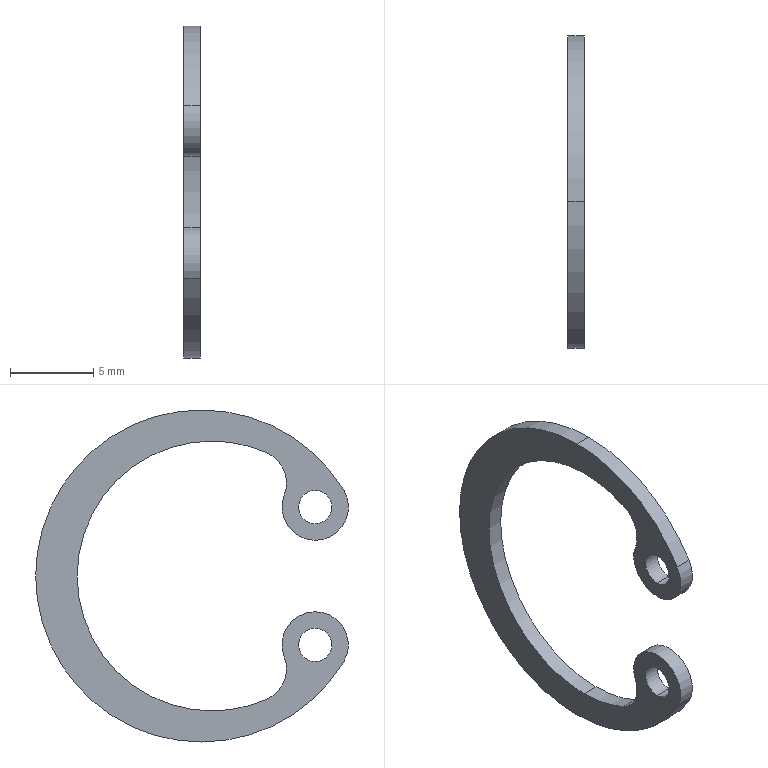Part | STEP file | _RTWN19 | 1 solid | 17 faces | box 1 x 18.839 x 20 mm | volume 110.311 mm3 | cylinder 15 | plane 2 | commonest cylinder face diameters 4 x5 2 x4 16.25 x3 20 x3
STEP:
#1=CARTESIAN_POINT('',(-0.5,-0.625,8.125));
#2=VERTEX_POINT('',#1);
#3=CARTESIAN_POINT('',(-0.5,-3.922,7.426));
#4=VERTEX_POINT('',#3);
#5=CARTESIAN_POINT('',(-0.5,-0.625,0.));
#6=DIRECTION('',(1.,0.,0.));
#7=DIRECTION('',(0.,0.,-1.));
#8=AXIS2_PLACEMENT_3D('',#5,#6,#7);
#9=CIRCLE('',#8,8.125);
#10=EDGE_CURVE('',#2,#4,#9,.T.);
#11=ORIENTED_EDGE('',*,*,#10,.F.);
#12=CARTESIAN_POINT('',(0.5,-0.625,8.125));
#13=VERTEX_POINT('',#12);
#14=CARTESIAN_POINT('',(0.5,-0.625,8.125));
#15=DIRECTION('',(1.,0.,0.));
#16=VECTOR('',#15,1000.);
#17=LINE('',#14,#16);
#18=EDGE_CURVE('',#2,#13,#17,.T.);
#19=ORIENTED_EDGE('',*,*,#18,.T.);
#20=CARTESIAN_POINT('',(0.5,-3.922,7.426));
#21=VERTEX_POINT('',#20);
#22=CARTESIAN_POINT('',(0.5,-0.625,0.));
#23=DIRECTION('',(-1.,0.,0.));
#24=DIRECTION('',(0.,0.,-1.));
#25=AXIS2_PLACEMENT_3D('',#22,#23,#24);
#26=CIRCLE('',#25,8.125);
#27=EDGE_CURVE('',#21,#13,#26,.T.);
#28=ORIENTED_EDGE('',*,*,#27,.F.);
#29=CARTESIAN_POINT('',(0.5,-3.922,7.426));
#30=DIRECTION('',(1.,0.,0.));
#31=VECTOR('',#30,1000.);
#32=LINE('',#29,#31);
#33=EDGE_CURVE('',#4,#21,#32,.T.);
#34=ORIENTED_EDGE('',*,*,#33,.F.);
#35=EDGE_LOOP('',(#11,#19,#28,#34));
#36=FACE_OUTER_BOUND('',#35,.T.);
#37=CARTESIAN_POINT('',(0.5,-0.625,0.));
#38=DIRECTION('',(1.,0.,0.));
#39=DIRECTION('',(0.,0.,-1.));
#40=AXIS2_PLACEMENT_3D('',#37,#38,#39);
#41=CYLINDRICAL_SURFACE('',#40,8.125);
#42=ADVANCED_FACE('',(#36),#41,.F.);
#43=ORIENTED_EDGE('',*,*,#18,.F.);
#44=CARTESIAN_POINT('',(-0.5,-0.625,-8.125));
#45=VERTEX_POINT('',#44);
#46=CARTESIAN_POINT('',(-0.5,-0.625,0.));
#47=DIRECTION('',(1.,0.,0.));
#48=DIRECTION('',(0.,0.,-1.));
#49=AXIS2_PLACEMENT_3D('',#46,#47,#48);
#50=CIRCLE('',#49,8.125);
#51=EDGE_CURVE('',#45,#2,#50,.T.);
#52=ORIENTED_EDGE('',*,*,#51,.F.);
#53=CARTESIAN_POINT('',(0.5,-0.625,-8.125));
#54=VERTEX_POINT('',#53);
#55=CARTESIAN_POINT('',(0.5,-0.625,-8.125));
#56=DIRECTION('',(1.,0.,0.));
#57=VECTOR('',#56,1000.);
#58=LINE('',#55,#57);
#59=EDGE_CURVE('',#45,#54,#58,.T.);
#60=ORIENTED_EDGE('',*,*,#59,.T.);
#61=CARTESIAN_POINT('',(0.5,-0.625,0.));
#62=DIRECTION('',(-1.,0.,0.));
#63=DIRECTION('',(0.,0.,-1.));
#64=AXIS2_PLACEMENT_3D('',#61,#62,#63);
#65=CIRCLE('',#64,8.125);
#66=EDGE_CURVE('',#13,#54,#65,.T.);
#67=ORIENTED_EDGE('',*,*,#66,.F.);
#68=EDGE_LOOP('',(#43,#52,#60,#67));
#69=FACE_OUTER_BOUND('',#68,.T.);
#70=CARTESIAN_POINT('',(0.5,-0.625,0.));
#71=DIRECTION('',(1.,0.,0.));
#72=DIRECTION('',(0.,0.,-1.));
#73=AXIS2_PLACEMENT_3D('',#70,#71,#72);
#74=CYLINDRICAL_SURFACE('',#73,8.125);
#75=ADVANCED_FACE('',(#69),#74,.F.);
#76=CARTESIAN_POINT('',(-0.5,-8.549,5.188));
#77=VERTEX_POINT('',#76);
#78=CARTESIAN_POINT('',(-0.5,-6.839,2.15));
#79=VERTEX_POINT('',#78);
#80=CARTESIAN_POINT('',(-0.5,-6.839,4.15));
#81=DIRECTION('',(1.,0.,0.));
#82=DIRECTION('',(0.,0.,-1.));
#83=AXIS2_PLACEMENT_3D('',#80,#81,#82);
#84=CIRCLE('',#83,2.);
#85=EDGE_CURVE('',#77,#79,#84,.T.);
#86=ORIENTED_EDGE('',*,*,#85,.T.);
#87=CARTESIAN_POINT('',(0.5,-6.839,2.15));
#88=VERTEX_POINT('',#87);
#89=CARTESIAN_POINT('',(0.5,-6.839,2.15));
#90=DIRECTION('',(1.,0.,0.));
#91=VECTOR('',#90,1000.);
#92=LINE('',#89,#91);
#93=EDGE_CURVE('',#79,#88,#92,.T.);
#94=ORIENTED_EDGE('',*,*,#93,.T.);
#95=CARTESIAN_POINT('',(0.5,-8.549,5.188));
#96=VERTEX_POINT('',#95);
#97=CARTESIAN_POINT('',(0.5,-6.839,4.15));
#98=DIRECTION('',(1.,0.,0.));
#99=DIRECTION('',(0.,0.,-1.));
#100=AXIS2_PLACEMENT_3D('',#97,#98,#99);
#101=CIRCLE('',#100,2.);
#102=EDGE_CURVE('',#96,#88,#101,.T.);
#103=ORIENTED_EDGE('',*,*,#102,.F.);
#104=CARTESIAN_POINT('',(0.5,-8.549,5.188));
#105=DIRECTION('',(-1.,0.,0.));
#106=VECTOR('',#105,1000.);
#107=LINE('',#104,#106);
#108=EDGE_CURVE('',#96,#77,#107,.T.);
#109=ORIENTED_EDGE('',*,*,#108,.T.);
#110=EDGE_LOOP('',(#86,#94,#103,#109));
#111=FACE_OUTER_BOUND('',#110,.T.);
#112=CARTESIAN_POINT('',(0.5,-6.839,4.15));
#113=DIRECTION('',(1.,0.,0.));
#114=DIRECTION('',(0.,0.,-1.));
#115=AXIS2_PLACEMENT_3D('',#112,#113,#114);
#116=CYLINDRICAL_SURFACE('',#115,2.);
#117=ADVANCED_FACE('',(#111),#116,.T.);
#118=CARTESIAN_POINT('',(-0.5,0.,-10.));
#119=VERTEX_POINT('',#118);
#120=CARTESIAN_POINT('',(-0.5,0.,10.));
#121=VERTEX_POINT('',#120);
#122=CARTESIAN_POINT('',(-0.5,0.,0.));
#123=DIRECTION('',(1.,0.,0.));
#124=DIRECTION('',(0.,0.,-1.));
#125=AXIS2_PLACEMENT_3D('',#122,#123,#124);
#126=CIRCLE('',#125,10.);
#127=EDGE_CURVE('',#119,#121,#126,.T.);
#128=ORIENTED_EDGE('',*,*,#127,.T.);
#129=CARTESIAN_POINT('',(0.5,0.,10.));
#130=VERTEX_POINT('',#129);
#131=CARTESIAN_POINT('',(0.5,0.,10.));
#132=DIRECTION('',(1.,0.,0.));
#133=VECTOR('',#132,1000.);
#134=LINE('',#131,#133);
#135=EDGE_CURVE('',#121,#130,#134,.T.);
#136=ORIENTED_EDGE('',*,*,#135,.T.);
#137=CARTESIAN_POINT('',(0.5,0.,-10.));
#138=VERTEX_POINT('',#137);
#139=CARTESIAN_POINT('',(0.5,0.,0.));
#140=DIRECTION('',(1.,0.,0.));
#141=DIRECTION('',(0.,0.,-1.));
#142=AXIS2_PLACEMENT_3D('',#139,#140,#141);
#143=CIRCLE('',#142,10.);
#144=EDGE_CURVE('',#138,#130,#143,.T.);
#145=ORIENTED_EDGE('',*,*,#144,.F.);
#146=CARTESIAN_POINT('',(0.5,0.,-10.));
#147=DIRECTION('',(1.,0.,0.));
#148=VECTOR('',#147,1000.);
#149=LINE('',#146,#148);
#150=EDGE_CURVE('',#119,#138,#149,.T.);
#151=ORIENTED_EDGE('',*,*,#150,.F.);
#152=EDGE_LOOP('',(#128,#136,#145,#151));
#153=FACE_OUTER_BOUND('',#152,.T.);
#154=CARTESIAN_POINT('',(0.5,0.,0.));
#155=DIRECTION('',(1.,0.,0.));
#156=DIRECTION('',(0.,0.,-1.));
#157=AXIS2_PLACEMENT_3D('',#154,#155,#156);
#158=CYLINDRICAL_SURFACE('',#157,10.);
#159=ADVANCED_FACE('',(#153),#158,.T.);
#160=CARTESIAN_POINT('',(-0.5,-8.549,-5.188));
#161=VERTEX_POINT('',#160);
#162=CARTESIAN_POINT('',(-0.5,0.,0.));
#163=DIRECTION('',(1.,0.,0.));
#164=DIRECTION('',(0.,0.,-1.));
#165=AXIS2_PLACEMENT_3D('',#162,#163,#164);
#166=CIRCLE('',#165,10.);
#167=EDGE_CURVE('',#161,#119,#166,.T.);
#168=ORIENTED_EDGE('',*,*,#167,.T.);
#169=ORIENTED_EDGE('',*,*,#150,.T.);
#170=CARTESIAN_POINT('',(0.5,-8.549,-5.188));
#171=VERTEX_POINT('',#170);
#172=CARTESIAN_POINT('',(0.5,0.,0.));
#173=DIRECTION('',(1.,0.,0.));
#174=DIRECTION('',(0.,0.,-1.));
#175=AXIS2_PLACEMENT_3D('',#172,#173,#174);
#176=CIRCLE('',#175,10.);
#177=EDGE_CURVE('',#171,#138,#176,.T.);
#178=ORIENTED_EDGE('',*,*,#177,.F.);
#179=CARTESIAN_POINT('',(0.5,-8.549,-5.187));
#180=DIRECTION('',(-1.,0.,0.));
#181=VECTOR('',#180,1000.);
#182=LINE('',#179,#181);
#183=EDGE_CURVE('',#171,#161,#182,.T.);
#184=ORIENTED_EDGE('',*,*,#183,.T.);
#185=EDGE_LOOP('',(#168,#169,#178,#184));
#186=FACE_OUTER_BOUND('',#185,.T.);
#187=CARTESIAN_POINT('',(0.5,0.,0.));
#188=DIRECTION('',(1.,0.,0.));
#189=DIRECTION('',(0.,0.,-1.));
#190=AXIS2_PLACEMENT_3D('',#187,#188,#189);
#191=CYLINDRICAL_SURFACE('',#190,10.);
#192=ADVANCED_FACE('',(#186),#191,.T.);
#193=CARTESIAN_POINT('',(-0.5,-6.839,-3.15));
#194=VERTEX_POINT('',#193);
#195=CARTESIAN_POINT('',(-0.5,-6.839,-5.15));
#196=VERTEX_POINT('',#195);
#197=CARTESIAN_POINT('',(-0.5,-6.839,-4.15));
#198=DIRECTION('',(1.,0.,0.));
#199=DIRECTION('',(0.,0.,-1.));
#200=AXIS2_PLACEMENT_3D('',#197,#198,#199);
#201=CIRCLE('',#200,1.);
#202=EDGE_CURVE('',#194,#196,#201,.T.);
#203=ORIENTED_EDGE('',*,*,#202,.F.);
#204=CARTESIAN_POINT('',(0.5,-6.839,-3.15));
#205=VERTEX_POINT('',#204);
#206=CARTESIAN_POINT('',(0.5,-6.839,-3.15));
#207=DIRECTION('',(1.,0.,0.));
#208=VECTOR('',#207,1000.);
#209=LINE('',#206,#208);
#210=EDGE_CURVE('',#194,#205,#209,.T.);
#211=ORIENTED_EDGE('',*,*,#210,.T.);
#212=CARTESIAN_POINT('',(0.5,-6.839,-5.15));
#213=VERTEX_POINT('',#212);
#214=CARTESIAN_POINT('',(0.5,-6.839,-4.15));
#215=DIRECTION('',(-1.,0.,0.));
#216=DIRECTION('',(0.,0.,-1.));
#217=AXIS2_PLACEMENT_3D('',#214,#215,#216);
#218=CIRCLE('',#217,1.);
#219=EDGE_CURVE('',#213,#205,#218,.T.);
#220=ORIENTED_EDGE('',*,*,#219,.F.);
#221=CARTESIAN_POINT('',(0.5,-6.839,-5.15));
#222=DIRECTION('',(1.,0.,0.));
#223=VECTOR('',#222,1000.);
#224=LINE('',#221,#223);
#225=EDGE_CURVE('',#196,#213,#224,.T.);
#226=ORIENTED_EDGE('',*,*,#225,.F.);
#227=EDGE_LOOP('',(#203,#211,#220,#226));
#228=FACE_OUTER_BOUND('',#227,.T.);
#229=CARTESIAN_POINT('',(0.5,-6.839,-4.15));
#230=DIRECTION('',(1.,0.,0.));
#231=DIRECTION('',(0.,0.,-1.));
#232=AXIS2_PLACEMENT_3D('',#229,#230,#231);
#233=CYLINDRICAL_SURFACE('',#232,1.);
#234=ADVANCED_FACE('',(#228),#233,.F.);
#235=CARTESIAN_POINT('',(-0.5,-6.839,5.15));
#236=VERTEX_POINT('',#235);
#237=CARTESIAN_POINT('',(-0.5,-6.839,3.15));
#238=VERTEX_POINT('',#237);
#239=CARTESIAN_POINT('',(-0.5,-6.839,4.15));
#240=DIRECTION('',(1.,0.,0.));
#241=DIRECTION('',(0.,0.,-1.));
#242=AXIS2_PLACEMENT_3D('',#239,#240,#241);
#243=CIRCLE('',#242,1.);
#244=EDGE_CURVE('',#236,#238,#243,.T.);
#245=ORIENTED_EDGE('',*,*,#244,.F.);
#246=CARTESIAN_POINT('',(0.5,-6.839,5.15));
#247=VERTEX_POINT('',#246);
#248=CARTESIAN_POINT('',(0.5,-6.839,5.15));
#249=DIRECTION('',(1.,0.,0.));
#250=VECTOR('',#249,1000.);
#251=LINE('',#248,#250);
#252=EDGE_CURVE('',#236,#247,#251,.T.);
#253=ORIENTED_EDGE('',*,*,#252,.T.);
#254=CARTESIAN_POINT('',(0.5,-6.839,3.15));
#255=VERTEX_POINT('',#254);
#256=CARTESIAN_POINT('',(0.5,-6.839,4.15));
#257=DIRECTION('',(-1.,0.,0.));
#258=DIRECTION('',(0.,0.,-1.));
#259=AXIS2_PLACEMENT_3D('',#256,#257,#258);
#260=CIRCLE('',#259,1.);
#261=EDGE_CURVE('',#255,#247,#260,.T.);
#262=ORIENTED_EDGE('',*,*,#261,.F.);
#263=CARTESIAN_POINT('',(0.5,-6.839,3.15));
#264=DIRECTION('',(1.,0.,0.));
#265=VECTOR('',#264,1000.);
#266=LINE('',#263,#265);
#267=EDGE_CURVE('',#238,#255,#266,.T.);
#268=ORIENTED_EDGE('',*,*,#267,.F.);
#269=EDGE_LOOP('',(#245,#253,#262,#268));
#270=FACE_OUTER_BOUND('',#269,.T.);
#271=CARTESIAN_POINT('',(0.5,-6.839,4.15));
#272=DIRECTION('',(1.,0.,0.));
#273=DIRECTION('',(0.,0.,-1.));
#274=AXIS2_PLACEMENT_3D('',#271,#272,#273);
#275=CYLINDRICAL_SURFACE('',#274,1.);
#276=ADVANCED_FACE('',(#270),#275,.F.);
#277=ORIENTED_EDGE('',*,*,#27,.T.);
#278=ORIENTED_EDGE('',*,*,#66,.T.);
#279=CARTESIAN_POINT('',(0.5,-3.922,-7.426));
#280=VERTEX_POINT('',#279);
#281=CARTESIAN_POINT('',(0.5,-0.625,0.));
#282=DIRECTION('',(-1.,0.,0.));
#283=DIRECTION('',(0.,0.,-1.));
#284=AXIS2_PLACEMENT_3D('',#281,#282,#283);
#285=CIRCLE('',#284,8.125);
#286=EDGE_CURVE('',#54,#280,#285,.T.);
#287=ORIENTED_EDGE('',*,*,#286,.T.);
#288=CARTESIAN_POINT('',(0.5,-4.975,-4.874));
#289=VERTEX_POINT('',#288);
#290=CARTESIAN_POINT('',(0.5,-3.111,-5.598));
#291=DIRECTION('',(-1.,0.,0.));
#292=DIRECTION('',(0.,0.,-1.));
#293=AXIS2_PLACEMENT_3D('',#290,#291,#292);
#294=CIRCLE('',#293,2.);
#295=EDGE_CURVE('',#280,#289,#294,.T.);
#296=ORIENTED_EDGE('',*,*,#295,.T.);
#297=CARTESIAN_POINT('',(0.5,-6.839,-4.15));
#298=DIRECTION('',(1.,0.,0.));
#299=DIRECTION('',(0.,0.,-1.));
#300=AXIS2_PLACEMENT_3D('',#297,#298,#299);
#301=CIRCLE('',#300,2.);
#302=EDGE_CURVE('',#289,#171,#301,.T.);
#303=ORIENTED_EDGE('',*,*,#302,.T.);
#304=ORIENTED_EDGE('',*,*,#177,.T.);
#305=ORIENTED_EDGE('',*,*,#144,.T.);
#306=CARTESIAN_POINT('',(0.5,0.,0.));
#307=DIRECTION('',(1.,0.,0.));
#308=DIRECTION('',(0.,0.,-1.));
#309=AXIS2_PLACEMENT_3D('',#306,#307,#308);
#310=CIRCLE('',#309,10.);
#311=EDGE_CURVE('',#130,#96,#310,.T.);
#312=ORIENTED_EDGE('',*,*,#311,.T.);
#313=ORIENTED_EDGE('',*,*,#102,.T.);
#314=CARTESIAN_POINT('',(0.5,-4.975,4.874));
#315=VERTEX_POINT('',#314);
#316=CARTESIAN_POINT('',(0.5,-6.839,4.15));
#317=DIRECTION('',(1.,0.,0.));
#318=DIRECTION('',(0.,0.,-1.));
#319=AXIS2_PLACEMENT_3D('',#316,#317,#318);
#320=CIRCLE('',#319,2.);
#321=EDGE_CURVE('',#88,#315,#320,.T.);
#322=ORIENTED_EDGE('',*,*,#321,.T.);
#323=CARTESIAN_POINT('',(0.5,-3.111,5.598));
#324=DIRECTION('',(-1.,0.,0.));
#325=DIRECTION('',(0.,0.,-1.));
#326=AXIS2_PLACEMENT_3D('',#323,#324,#325);
#327=CIRCLE('',#326,2.);
#328=EDGE_CURVE('',#315,#21,#327,.T.);
#329=ORIENTED_EDGE('',*,*,#328,.T.);
#330=EDGE_LOOP('',(#277,#278,#287,#296,#303,#304,#305,#312,#313,#322,#329));
#331=FACE_OUTER_BOUND('',#330,.T.);
#332=ORIENTED_EDGE('',*,*,#219,.T.);
#333=CARTESIAN_POINT('',(0.5,-6.839,-4.15));
#334=DIRECTION('',(-1.,0.,0.));
#335=DIRECTION('',(0.,0.,-1.));
#336=AXIS2_PLACEMENT_3D('',#333,#334,#335);
#337=CIRCLE('',#336,1.);
#338=EDGE_CURVE('',#205,#213,#337,.T.);
#339=ORIENTED_EDGE('',*,*,#338,.T.);
#340=EDGE_LOOP('',(#332,#339));
#341=FACE_BOUND('',#340,.T.);
#342=ORIENTED_EDGE('',*,*,#261,.T.);
#343=CARTESIAN_POINT('',(0.5,-6.839,4.15));
#344=DIRECTION('',(-1.,0.,0.));
#345=DIRECTION('',(0.,0.,-1.));
#346=AXIS2_PLACEMENT_3D('',#343,#344,#345);
#347=CIRCLE('',#346,1.);
#348=EDGE_CURVE('',#247,#255,#347,.T.);
#349=ORIENTED_EDGE('',*,*,#348,.T.);
#350=EDGE_LOOP('',(#342,#349));
#351=FACE_BOUND('',#350,.T.);
#352=CARTESIAN_POINT('',(0.5,-3.42,-2.075));
#353=DIRECTION('',(1.,0.,0.));
#354=DIRECTION('',(0.,0.,-1.));
#355=AXIS2_PLACEMENT_3D('',#352,#353,#354);
#356=PLANE('',#355);
#357=ADVANCED_FACE('',(#331,#341,#351),#356,.T.);
#358=CARTESIAN_POINT('',(-0.5,-4.975,-4.874));
#359=VERTEX_POINT('',#358);
#360=CARTESIAN_POINT('',(0.5,-4.975,-4.874));
#361=DIRECTION('',(-1.,0.,0.));
#362=VECTOR('',#361,1000.);
#363=LINE('',#360,#362);
#364=EDGE_CURVE('',#289,#359,#363,.T.);
#365=ORIENTED_EDGE('',*,*,#364,.F.);
#366=ORIENTED_EDGE('',*,*,#295,.F.);
#367=CARTESIAN_POINT('',(-0.5,-3.922,-7.426));
#368=VERTEX_POINT('',#367);
#369=CARTESIAN_POINT('',(0.5,-3.922,-7.426));
#370=DIRECTION('',(1.,0.,0.));
#371=VECTOR('',#370,1000.);
#372=LINE('',#369,#371);
#373=EDGE_CURVE('',#368,#280,#372,.T.);
#374=ORIENTED_EDGE('',*,*,#373,.F.);
#375=CARTESIAN_POINT('',(-0.5,-3.111,-5.598));
#376=DIRECTION('',(1.,0.,0.));
#377=DIRECTION('',(0.,0.,-1.));
#378=AXIS2_PLACEMENT_3D('',#375,#376,#377);
#379=CIRCLE('',#378,2.);
#380=EDGE_CURVE('',#359,#368,#379,.T.);
#381=ORIENTED_EDGE('',*,*,#380,.F.);
#382=EDGE_LOOP('',(#365,#366,#374,#381));
#383=FACE_OUTER_BOUND('',#382,.T.);
#384=CARTESIAN_POINT('',(0.5,-3.111,-5.598));
#385=DIRECTION('',(1.,0.,0.));
#386=DIRECTION('',(0.,0.,-1.));
#387=AXIS2_PLACEMENT_3D('',#384,#385,#386);
#388=CYLINDRICAL_SURFACE('',#387,2.);
#389=ADVANCED_FACE('',(#383),#388,.F.);
#390=ORIENTED_EDGE('',*,*,#59,.F.);
#391=CARTESIAN_POINT('',(-0.5,-0.625,0.));
#392=DIRECTION('',(1.,0.,0.));
#393=DIRECTION('',(0.,0.,-1.));
#394=AXIS2_PLACEMENT_3D('',#391,#392,#393);
#395=CIRCLE('',#394,8.125);
#396=EDGE_CURVE('',#368,#45,#395,.T.);
#397=ORIENTED_EDGE('',*,*,#396,.F.);
#398=ORIENTED_EDGE('',*,*,#373,.T.);
#399=ORIENTED_EDGE('',*,*,#286,.F.);
#400=EDGE_LOOP('',(#390,#397,#398,#399));
#401=FACE_OUTER_BOUND('',#400,.T.);
#402=CARTESIAN_POINT('',(0.5,-0.625,0.));
#403=DIRECTION('',(1.,0.,0.));
#404=DIRECTION('',(0.,0.,-1.));
#405=AXIS2_PLACEMENT_3D('',#402,#403,#404);
#406=CYLINDRICAL_SURFACE('',#405,8.125);
#407=ADVANCED_FACE('',(#401),#406,.F.);
#408=ORIENTED_EDGE('',*,*,#33,.T.);
#409=ORIENTED_EDGE('',*,*,#328,.F.);
#410=CARTESIAN_POINT('',(-0.5,-4.975,4.874));
#411=VERTEX_POINT('',#410);
#412=CARTESIAN_POINT('',(0.5,-4.975,4.874));
#413=DIRECTION('',(1.,0.,0.));
#414=VECTOR('',#413,1000.);
#415=LINE('',#412,#414);
#416=EDGE_CURVE('',#411,#315,#415,.T.);
#417=ORIENTED_EDGE('',*,*,#416,.F.);
#418=CARTESIAN_POINT('',(-0.5,-3.111,5.598));
#419=DIRECTION('',(1.,0.,0.));
#420=DIRECTION('',(0.,0.,-1.));
#421=AXIS2_PLACEMENT_3D('',#418,#419,#420);
#422=CIRCLE('',#421,2.);
#423=EDGE_CURVE('',#4,#411,#422,.T.);
#424=ORIENTED_EDGE('',*,*,#423,.F.);
#425=EDGE_LOOP('',(#408,#409,#417,#424));
#426=FACE_OUTER_BOUND('',#425,.T.);
#427=CARTESIAN_POINT('',(0.5,-3.111,5.598));
#428=DIRECTION('',(1.,0.,0.));
#429=DIRECTION('',(0.,0.,-1.));
#430=AXIS2_PLACEMENT_3D('',#427,#428,#429);
#431=CYLINDRICAL_SURFACE('',#430,2.);
#432=ADVANCED_FACE('',(#426),#431,.F.);
#433=ORIENTED_EDGE('',*,*,#93,.F.);
#434=CARTESIAN_POINT('',(-0.5,-6.839,4.15));
#435=DIRECTION('',(1.,0.,0.));
#436=DIRECTION('',(0.,0.,-1.));
#437=AXIS2_PLACEMENT_3D('',#434,#435,#436);
#438=CIRCLE('',#437,2.);
#439=EDGE_CURVE('',#79,#411,#438,.T.);
#440=ORIENTED_EDGE('',*,*,#439,.T.);
#441=ORIENTED_EDGE('',*,*,#416,.T.);
#442=ORIENTED_EDGE('',*,*,#321,.F.);
#443=EDGE_LOOP('',(#433,#440,#441,#442));
#444=FACE_OUTER_BOUND('',#443,.T.);
#445=CARTESIAN_POINT('',(0.5,-6.839,4.15));
#446=DIRECTION('',(1.,0.,0.));
#447=DIRECTION('',(0.,0.,-1.));
#448=AXIS2_PLACEMENT_3D('',#445,#446,#447);
#449=CYLINDRICAL_SURFACE('',#448,2.);
#450=ADVANCED_FACE('',(#444),#449,.T.);
#451=ORIENTED_EDGE('',*,*,#135,.F.);
#452=CARTESIAN_POINT('',(-0.5,0.,0.));
#453=DIRECTION('',(1.,0.,0.));
#454=DIRECTION('',(0.,0.,-1.));
#455=AXIS2_PLACEMENT_3D('',#452,#453,#454);
#456=CIRCLE('',#455,10.);
#457=EDGE_CURVE('',#121,#77,#456,.T.);
#458=ORIENTED_EDGE('',*,*,#457,.T.);
#459=ORIENTED_EDGE('',*,*,#108,.F.);
#460=ORIENTED_EDGE('',*,*,#311,.F.);
#461=EDGE_LOOP('',(#451,#458,#459,#460));
#462=FACE_OUTER_BOUND('',#461,.T.);
#463=CARTESIAN_POINT('',(0.5,0.,0.));
#464=DIRECTION('',(1.,0.,0.));
#465=DIRECTION('',(0.,0.,-1.));
#466=AXIS2_PLACEMENT_3D('',#463,#464,#465);
#467=CYLINDRICAL_SURFACE('',#466,10.);
#468=ADVANCED_FACE('',(#462),#467,.T.);
#469=ORIENTED_EDGE('',*,*,#302,.F.);
#470=ORIENTED_EDGE('',*,*,#364,.T.);
#471=CARTESIAN_POINT('',(-0.5,-6.839,-4.15));
#472=DIRECTION('',(1.,0.,0.));
#473=DIRECTION('',(0.,0.,-1.));
#474=AXIS2_PLACEMENT_3D('',#471,#472,#473);
#475=CIRCLE('',#474,2.);
#476=EDGE_CURVE('',#359,#161,#475,.T.);
#477=ORIENTED_EDGE('',*,*,#476,.T.);
#478=ORIENTED_EDGE('',*,*,#183,.F.);
#479=EDGE_LOOP('',(#469,#470,#477,#478));
#480=FACE_OUTER_BOUND('',#479,.T.);
#481=CARTESIAN_POINT('',(0.5,-6.839,-4.15));
#482=DIRECTION('',(1.,0.,0.));
#483=DIRECTION('',(0.,0.,-1.));
#484=AXIS2_PLACEMENT_3D('',#481,#482,#483);
#485=CYLINDRICAL_SURFACE('',#484,2.);
#486=ADVANCED_FACE('',(#480),#485,.T.);
#487=ORIENTED_EDGE('',*,*,#210,.F.);
#488=CARTESIAN_POINT('',(-0.5,-6.839,-4.15));
#489=DIRECTION('',(1.,0.,0.));
#490=DIRECTION('',(0.,0.,-1.));
#491=AXIS2_PLACEMENT_3D('',#488,#489,#490);
#492=CIRCLE('',#491,1.);
#493=EDGE_CURVE('',#196,#194,#492,.T.);
#494=ORIENTED_EDGE('',*,*,#493,.F.);
#495=ORIENTED_EDGE('',*,*,#225,.T.);
#496=ORIENTED_EDGE('',*,*,#338,.F.);
#497=EDGE_LOOP('',(#487,#494,#495,#496));
#498=FACE_OUTER_BOUND('',#497,.T.);
#499=CARTESIAN_POINT('',(0.5,-6.839,-4.15));
#500=DIRECTION('',(1.,0.,0.));
#501=DIRECTION('',(0.,0.,-1.));
#502=AXIS2_PLACEMENT_3D('',#499,#500,#501);
#503=CYLINDRICAL_SURFACE('',#502,1.);
#504=ADVANCED_FACE('',(#498),#503,.F.);
#505=ORIENTED_EDGE('',*,*,#252,.F.);
#506=CARTESIAN_POINT('',(-0.5,-6.839,4.15));
#507=DIRECTION('',(1.,0.,0.));
#508=DIRECTION('',(0.,0.,-1.));
#509=AXIS2_PLACEMENT_3D('',#506,#507,#508);
#510=CIRCLE('',#509,1.);
#511=EDGE_CURVE('',#238,#236,#510,.T.);
#512=ORIENTED_EDGE('',*,*,#511,.F.);
#513=ORIENTED_EDGE('',*,*,#267,.T.);
#514=ORIENTED_EDGE('',*,*,#348,.F.);
#515=EDGE_LOOP('',(#505,#512,#513,#514));
#516=FACE_OUTER_BOUND('',#515,.T.);
#517=CARTESIAN_POINT('',(0.5,-6.839,4.15));
#518=DIRECTION('',(1.,0.,0.));
#519=DIRECTION('',(0.,0.,-1.));
#520=AXIS2_PLACEMENT_3D('',#517,#518,#519);
#521=CYLINDRICAL_SURFACE('',#520,1.);
#522=ADVANCED_FACE('',(#516),#521,.F.);
#523=ORIENTED_EDGE('',*,*,#476,.F.);
#524=ORIENTED_EDGE('',*,*,#380,.T.);
#525=ORIENTED_EDGE('',*,*,#396,.T.);
#526=ORIENTED_EDGE('',*,*,#51,.T.);
#527=ORIENTED_EDGE('',*,*,#10,.T.);
#528=ORIENTED_EDGE('',*,*,#423,.T.);
#529=ORIENTED_EDGE('',*,*,#439,.F.);
#530=ORIENTED_EDGE('',*,*,#85,.F.);
#531=ORIENTED_EDGE('',*,*,#457,.F.);
#532=ORIENTED_EDGE('',*,*,#127,.F.);
#533=ORIENTED_EDGE('',*,*,#167,.F.);
#534=EDGE_LOOP('',(#523,#524,#525,#526,#527,#528,#529,#530,#531,#532,#533));
#535=FACE_OUTER_BOUND('',#534,.T.);
#536=ORIENTED_EDGE('',*,*,#493,.T.);
#537=ORIENTED_EDGE('',*,*,#202,.T.);
#538=EDGE_LOOP('',(#536,#537));
#539=FACE_BOUND('',#538,.T.);
#540=ORIENTED_EDGE('',*,*,#511,.T.);
#541=ORIENTED_EDGE('',*,*,#244,.T.);
#542=EDGE_LOOP('',(#540,#541));
#543=FACE_BOUND('',#542,.T.);
#544=CARTESIAN_POINT('',(-0.5,-3.42,-2.075));
#545=DIRECTION('',(1.,0.,0.));
#546=DIRECTION('',(0.,0.,-1.));
#547=AXIS2_PLACEMENT_3D('',#544,#545,#546);
#548=PLANE('',#547);
#549=ADVANCED_FACE('',(#535,#539,#543),#548,.F.);
#550=CLOSED_SHELL('',(#42,#75,#117,#159,#192,#234,#276,#357,#389,#407,#432,#450,#468,#486,#504,#522,#549));
#551=MANIFOLD_SOLID_BREP('',#550);
#552=CARTESIAN_POINT('',(0.,0.,0.));
#553=DIRECTION('',(0.,0.,1.));
#554=DIRECTION('',(1.,0.,0.));
#555=AXIS2_PLACEMENT_3D('',#552,#553,#554);
#556=(LENGTH_UNIT()NAMED_UNIT(*)SI_UNIT(.MILLI.,.METRE.));
#557=UNCERTAINTY_MEASURE_WITH_UNIT(LENGTH_MEASURE(0.00001),#556,'','');
#558=(NAMED_UNIT(*)PLANE_ANGLE_UNIT()SI_UNIT($,.RADIAN.));
#559=(NAMED_UNIT(*)SI_UNIT($,.STERADIAN.)SOLID_ANGLE_UNIT());
#560=(GEOMETRIC_REPRESENTATION_CONTEXT(3)GLOBAL_UNCERTAINTY_ASSIGNED_CONTEXT((#557))GLOBAL_UNIT_ASSIGNED_CONTEXT((#556,#558,#559))REPRESENTATION_CONTEXT('',''));
#561=ADVANCED_BREP_SHAPE_REPRESENTATION('',(#551,#555),#560);